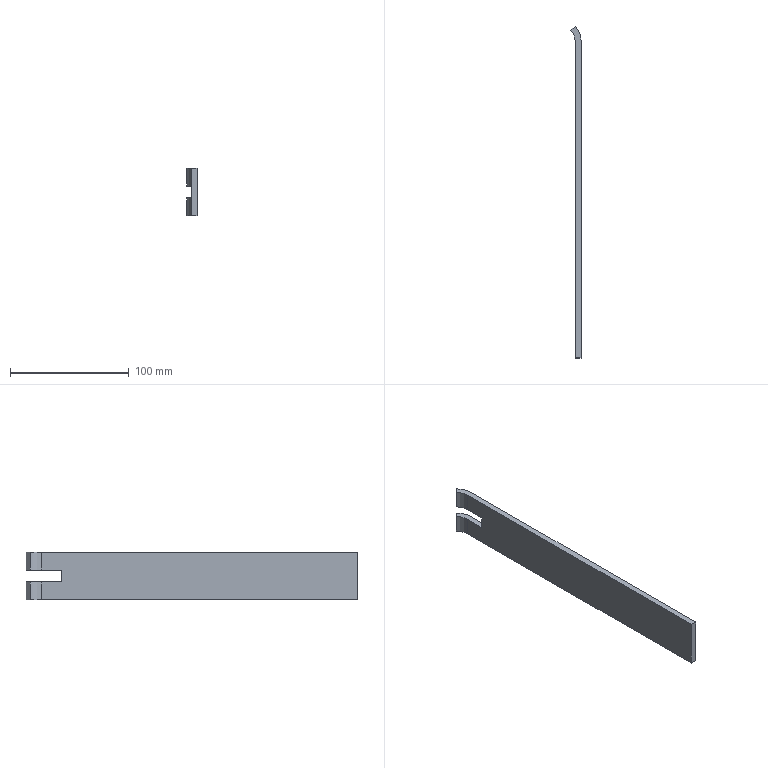Part | SolidWorks | features ICE 2, Extrusion 1 | 1 solid | 14 faces | box 8.684 x 279.845 x 40 mm | volume 54380 mm3 | plane 10 | cylinder 4 | commonest cylinder face diameters 28 x2 38 x2
STEP:
#1=CARTESIAN_POINT('',(0.,273.845,15.));
#2=VERTEX_POINT('',#1);
#3=CARTESIAN_POINT('',(0.,273.845,0.));
#4=VERTEX_POINT('',#3);
#5=CARTESIAN_POINT('',(0.,273.845,40.));
#6=DIRECTION('',(0.,0.,-1.));
#7=VECTOR('',#6,1000.);
#8=LINE('',#5,#7);
#9=EDGE_CURVE('',#2,#4,#8,.T.);
#10=ORIENTED_EDGE('',*,*,#9,.F.);
#11=CARTESIAN_POINT('',(5.,261.,15.));
#12=VERTEX_POINT('',#11);
#13=CARTESIAN_POINT('',(-14.,261.,15.));
#14=DIRECTION('',(0.,0.,-1.));
#15=DIRECTION('',(0.,1.,0.));
#16=AXIS2_PLACEMENT_3D('',#13,#14,#15);
#17=CIRCLE('',#16,19.);
#18=EDGE_CURVE('',#2,#12,#17,.T.);
#19=ORIENTED_EDGE('',*,*,#18,.T.);
#20=CARTESIAN_POINT('',(5.,261.,0.));
#21=VERTEX_POINT('',#20);
#22=CARTESIAN_POINT('',(5.,261.,40.));
#23=DIRECTION('',(0.,0.,-1.));
#24=VECTOR('',#23,1000.);
#25=LINE('',#22,#24);
#26=EDGE_CURVE('',#12,#21,#25,.T.);
#27=ORIENTED_EDGE('',*,*,#26,.T.);
#28=CARTESIAN_POINT('',(-14.,261.,0.));
#29=DIRECTION('',(0.,0.,1.));
#30=DIRECTION('',(1.,0.,0.));
#31=AXIS2_PLACEMENT_3D('',#28,#29,#30);
#32=CIRCLE('',#31,19.);
#33=EDGE_CURVE('',#21,#4,#32,.T.);
#34=ORIENTED_EDGE('',*,*,#33,.T.);
#35=EDGE_LOOP('',(#10,#19,#27,#34));
#36=FACE_OUTER_BOUND('',#35,.T.);
#37=CARTESIAN_POINT('',(-14.,261.,40.));
#38=DIRECTION('',(0.,0.,-1.));
#39=DIRECTION('',(-1.,0.,0.));
#40=AXIS2_PLACEMENT_3D('',#37,#38,#39);
#41=CYLINDRICAL_SURFACE('',#40,19.);
#42=ADVANCED_FACE('',(#36),#41,.T.);
#43=CARTESIAN_POINT('',(-3.684,270.465,15.));
#44=VERTEX_POINT('',#43);
#45=CARTESIAN_POINT('',(-3.684,270.465,0.));
#46=VERTEX_POINT('',#45);
#47=CARTESIAN_POINT('',(-3.684,270.465,40.));
#48=DIRECTION('',(0.,0.,-1.));
#49=VECTOR('',#48,1000.);
#50=LINE('',#47,#49);
#51=EDGE_CURVE('',#44,#46,#50,.T.);
#52=ORIENTED_EDGE('',*,*,#51,.F.);
#53=CARTESIAN_POINT('',(-3.684,270.465,15.));
#54=DIRECTION('',(0.7368,0.6761,0.));
#55=VECTOR('',#54,1000.);
#56=LINE('',#53,#55);
#57=EDGE_CURVE('',#44,#2,#56,.T.);
#58=ORIENTED_EDGE('',*,*,#57,.T.);
#59=ORIENTED_EDGE('',*,*,#9,.T.);
#60=CARTESIAN_POINT('',(-3.684,270.465,0.));
#61=DIRECTION('',(-0.7368,-0.6761,0.));
#62=VECTOR('',#61,1000.);
#63=LINE('',#60,#62);
#64=EDGE_CURVE('',#4,#46,#63,.T.);
#65=ORIENTED_EDGE('',*,*,#64,.T.);
#66=EDGE_LOOP('',(#52,#58,#59,#65));
#67=FACE_OUTER_BOUND('',#66,.T.);
#68=CARTESIAN_POINT('',(-3.684,270.465,40.));
#69=DIRECTION('',(0.6761,-0.7368,0.));
#70=DIRECTION('',(0.7368,0.6761,0.));
#71=AXIS2_PLACEMENT_3D('',#68,#69,#70);
#72=PLANE('',#71);
#73=ADVANCED_FACE('',(#67),#72,.F.);
#74=CARTESIAN_POINT('',(0.,261.,15.));
#75=VERTEX_POINT('',#74);
#76=CARTESIAN_POINT('',(0.,261.,0.));
#77=VERTEX_POINT('',#76);
#78=CARTESIAN_POINT('',(0.,261.,40.));
#79=DIRECTION('',(0.,0.,-1.));
#80=VECTOR('',#79,1000.);
#81=LINE('',#78,#80);
#82=EDGE_CURVE('',#75,#77,#81,.T.);
#83=ORIENTED_EDGE('',*,*,#82,.F.);
#84=CARTESIAN_POINT('',(-14.,261.,15.));
#85=DIRECTION('',(0.,0.,1.));
#86=DIRECTION('',(0.,1.,0.));
#87=AXIS2_PLACEMENT_3D('',#84,#85,#86);
#88=CIRCLE('',#87,14.);
#89=EDGE_CURVE('',#75,#44,#88,.T.);
#90=ORIENTED_EDGE('',*,*,#89,.T.);
#91=ORIENTED_EDGE('',*,*,#51,.T.);
#92=CARTESIAN_POINT('',(-14.,261.,0.));
#93=DIRECTION('',(0.,0.,-1.));
#94=DIRECTION('',(1.,0.,0.));
#95=AXIS2_PLACEMENT_3D('',#92,#93,#94);
#96=CIRCLE('',#95,14.);
#97=EDGE_CURVE('',#46,#77,#96,.T.);
#98=ORIENTED_EDGE('',*,*,#97,.T.);
#99=EDGE_LOOP('',(#83,#90,#91,#98));
#100=FACE_OUTER_BOUND('',#99,.T.);
#101=CARTESIAN_POINT('',(-14.,261.,40.));
#102=DIRECTION('',(0.,0.,-1.));
#103=DIRECTION('',(-1.,0.,0.));
#104=AXIS2_PLACEMENT_3D('',#101,#102,#103);
#105=CYLINDRICAL_SURFACE('',#104,14.);
#106=ADVANCED_FACE('',(#100),#105,.F.);
#107=CARTESIAN_POINT('',(0.,243.845,25.));
#108=VERTEX_POINT('',#107);
#109=CARTESIAN_POINT('',(0.,243.845,15.));
#110=VERTEX_POINT('',#109);
#111=CARTESIAN_POINT('',(0.,243.845,40.));
#112=DIRECTION('',(0.,0.,-1.));
#113=VECTOR('',#112,1000.);
#114=LINE('',#111,#113);
#115=EDGE_CURVE('',#108,#110,#114,.T.);
#116=ORIENTED_EDGE('',*,*,#115,.T.);
#117=CARTESIAN_POINT('',(0.,0.,15.));
#118=DIRECTION('',(0.,1.,0.));
#119=VECTOR('',#118,1000.);
#120=LINE('',#117,#119);
#121=EDGE_CURVE('',#110,#75,#120,.T.);
#122=ORIENTED_EDGE('',*,*,#121,.T.);
#123=ORIENTED_EDGE('',*,*,#82,.T.);
#124=CARTESIAN_POINT('',(0.,-6.,0.));
#125=VERTEX_POINT('',#124);
#126=CARTESIAN_POINT('',(0.,0.,0.));
#127=DIRECTION('',(0.,-1.,0.));
#128=VECTOR('',#127,1000.);
#129=LINE('',#126,#128);
#130=EDGE_CURVE('',#77,#125,#129,.T.);
#131=ORIENTED_EDGE('',*,*,#130,.T.);
#132=CARTESIAN_POINT('',(0.,-6.,40.));
#133=VERTEX_POINT('',#132);
#134=CARTESIAN_POINT('',(0.,-6.,40.));
#135=DIRECTION('',(0.,0.,-1.));
#136=VECTOR('',#135,1000.);
#137=LINE('',#134,#136);
#138=EDGE_CURVE('',#133,#125,#137,.T.);
#139=ORIENTED_EDGE('',*,*,#138,.F.);
#140=CARTESIAN_POINT('',(0.,261.,40.));
#141=VERTEX_POINT('',#140);
#142=CARTESIAN_POINT('',(0.,0.,40.));
#143=DIRECTION('',(0.,-1.,0.));
#144=VECTOR('',#143,1000.);
#145=LINE('',#142,#144);
#146=EDGE_CURVE('',#141,#133,#145,.T.);
#147=ORIENTED_EDGE('',*,*,#146,.F.);
#148=CARTESIAN_POINT('',(0.,261.,25.));
#149=VERTEX_POINT('',#148);
#150=CARTESIAN_POINT('',(0.,261.,40.));
#151=DIRECTION('',(0.,0.,-1.));
#152=VECTOR('',#151,1000.);
#153=LINE('',#150,#152);
#154=EDGE_CURVE('',#141,#149,#153,.T.);
#155=ORIENTED_EDGE('',*,*,#154,.T.);
#156=CARTESIAN_POINT('',(0.,0.,25.));
#157=DIRECTION('',(0.,-1.,0.));
#158=VECTOR('',#157,1000.);
#159=LINE('',#156,#158);
#160=EDGE_CURVE('',#149,#108,#159,.T.);
#161=ORIENTED_EDGE('',*,*,#160,.T.);
#162=EDGE_LOOP('',(#116,#122,#123,#131,#139,#147,#155,#161));
#163=FACE_OUTER_BOUND('',#162,.T.);
#164=CARTESIAN_POINT('',(0.,0.,40.));
#165=DIRECTION('',(1.,0.,0.));
#166=DIRECTION('',(0.,1.,0.));
#167=AXIS2_PLACEMENT_3D('',#164,#165,#166);
#168=PLANE('',#167);
#169=ADVANCED_FACE('',(#163),#168,.F.);
#170=ORIENTED_EDGE('',*,*,#26,.F.);
#171=CARTESIAN_POINT('',(5.,243.845,15.));
#172=VERTEX_POINT('',#171);
#173=CARTESIAN_POINT('',(5.,273.845,15.));
#174=DIRECTION('',(0.,1.,0.));
#175=VECTOR('',#174,1000.);
#176=LINE('',#173,#175);
#177=EDGE_CURVE('',#172,#12,#176,.T.);
#178=ORIENTED_EDGE('',*,*,#177,.F.);
#179=CARTESIAN_POINT('',(5.,243.845,25.));
#180=VERTEX_POINT('',#179);
#181=CARTESIAN_POINT('',(5.,243.845,15.));
#182=DIRECTION('',(0.,0.,-1.));
#183=VECTOR('',#182,1000.);
#184=LINE('',#181,#183);
#185=EDGE_CURVE('',#180,#172,#184,.T.);
#186=ORIENTED_EDGE('',*,*,#185,.F.);
#187=CARTESIAN_POINT('',(5.,261.,25.));
#188=VERTEX_POINT('',#187);
#189=CARTESIAN_POINT('',(5.,243.845,25.));
#190=DIRECTION('',(0.,-1.,0.));
#191=VECTOR('',#190,1000.);
#192=LINE('',#189,#191);
#193=EDGE_CURVE('',#188,#180,#192,.T.);
#194=ORIENTED_EDGE('',*,*,#193,.F.);
#195=CARTESIAN_POINT('',(5.,261.,40.));
#196=VERTEX_POINT('',#195);
#197=CARTESIAN_POINT('',(5.,261.,40.));
#198=DIRECTION('',(0.,0.,-1.));
#199=VECTOR('',#198,1000.);
#200=LINE('',#197,#199);
#201=EDGE_CURVE('',#196,#188,#200,.T.);
#202=ORIENTED_EDGE('',*,*,#201,.F.);
#203=CARTESIAN_POINT('',(5.,-6.,40.));
#204=VERTEX_POINT('',#203);
#205=CARTESIAN_POINT('',(5.,0.,40.));
#206=DIRECTION('',(0.,1.,0.));
#207=VECTOR('',#206,1000.);
#208=LINE('',#205,#207);
#209=EDGE_CURVE('',#204,#196,#208,.T.);
#210=ORIENTED_EDGE('',*,*,#209,.F.);
#211=CARTESIAN_POINT('',(5.,-6.,0.));
#212=VERTEX_POINT('',#211);
#213=CARTESIAN_POINT('',(5.,-6.,0.));
#214=DIRECTION('',(0.,0.,1.));
#215=VECTOR('',#214,1000.);
#216=LINE('',#213,#215);
#217=EDGE_CURVE('',#212,#204,#216,.T.);
#218=ORIENTED_EDGE('',*,*,#217,.F.);
#219=CARTESIAN_POINT('',(5.,0.,0.));
#220=DIRECTION('',(0.,1.,0.));
#221=VECTOR('',#220,1000.);
#222=LINE('',#219,#221);
#223=EDGE_CURVE('',#212,#21,#222,.T.);
#224=ORIENTED_EDGE('',*,*,#223,.T.);
#225=EDGE_LOOP('',(#170,#178,#186,#194,#202,#210,#218,#224));
#226=FACE_OUTER_BOUND('',#225,.T.);
#227=CARTESIAN_POINT('',(5.,0.,40.));
#228=DIRECTION('',(-1.,0.,0.));
#229=DIRECTION('',(0.,0.,1.));
#230=AXIS2_PLACEMENT_3D('',#227,#228,#229);
#231=PLANE('',#230);
#232=ADVANCED_FACE('',(#226),#231,.F.);
#233=ORIENTED_EDGE('',*,*,#201,.T.);
#234=CARTESIAN_POINT('',(0.,273.845,25.));
#235=VERTEX_POINT('',#234);
#236=CARTESIAN_POINT('',(-14.,261.,25.));
#237=DIRECTION('',(0.,0.,1.));
#238=DIRECTION('',(1.,0.,0.));
#239=AXIS2_PLACEMENT_3D('',#236,#237,#238);
#240=CIRCLE('',#239,19.);
#241=EDGE_CURVE('',#188,#235,#240,.T.);
#242=ORIENTED_EDGE('',*,*,#241,.T.);
#243=CARTESIAN_POINT('',(0.,273.845,40.));
#244=VERTEX_POINT('',#243);
#245=CARTESIAN_POINT('',(0.,273.845,40.));
#246=DIRECTION('',(0.,0.,-1.));
#247=VECTOR('',#246,1000.);
#248=LINE('',#245,#247);
#249=EDGE_CURVE('',#244,#235,#248,.T.);
#250=ORIENTED_EDGE('',*,*,#249,.F.);
#251=CARTESIAN_POINT('',(-14.,261.,40.));
#252=DIRECTION('',(0.,0.,1.));
#253=DIRECTION('',(1.,0.,0.));
#254=AXIS2_PLACEMENT_3D('',#251,#252,#253);
#255=CIRCLE('',#254,19.);
#256=EDGE_CURVE('',#196,#244,#255,.T.);
#257=ORIENTED_EDGE('',*,*,#256,.F.);
#258=EDGE_LOOP('',(#233,#242,#250,#257));
#259=FACE_OUTER_BOUND('',#258,.T.);
#260=CARTESIAN_POINT('',(-14.,261.,40.));
#261=DIRECTION('',(0.,0.,-1.));
#262=DIRECTION('',(-1.,0.,0.));
#263=AXIS2_PLACEMENT_3D('',#260,#261,#262);
#264=CYLINDRICAL_SURFACE('',#263,19.);
#265=ADVANCED_FACE('',(#259),#264,.T.);
#266=ORIENTED_EDGE('',*,*,#249,.T.);
#267=CARTESIAN_POINT('',(-3.684,270.465,25.));
#268=VERTEX_POINT('',#267);
#269=CARTESIAN_POINT('',(-3.684,270.465,25.));
#270=DIRECTION('',(-0.7368,-0.6761,0.));
#271=VECTOR('',#270,1000.);
#272=LINE('',#269,#271);
#273=EDGE_CURVE('',#235,#268,#272,.T.);
#274=ORIENTED_EDGE('',*,*,#273,.T.);
#275=CARTESIAN_POINT('',(-3.684,270.465,40.));
#276=VERTEX_POINT('',#275);
#277=CARTESIAN_POINT('',(-3.684,270.465,40.));
#278=DIRECTION('',(0.,0.,-1.));
#279=VECTOR('',#278,1000.);
#280=LINE('',#277,#279);
#281=EDGE_CURVE('',#276,#268,#280,.T.);
#282=ORIENTED_EDGE('',*,*,#281,.F.);
#283=CARTESIAN_POINT('',(-3.684,270.465,40.));
#284=DIRECTION('',(-0.7368,-0.6761,0.));
#285=VECTOR('',#284,1000.);
#286=LINE('',#283,#285);
#287=EDGE_CURVE('',#244,#276,#286,.T.);
#288=ORIENTED_EDGE('',*,*,#287,.F.);
#289=EDGE_LOOP('',(#266,#274,#282,#288));
#290=FACE_OUTER_BOUND('',#289,.T.);
#291=CARTESIAN_POINT('',(-3.684,270.465,40.));
#292=DIRECTION('',(0.6761,-0.7368,0.));
#293=DIRECTION('',(0.7368,0.6761,0.));
#294=AXIS2_PLACEMENT_3D('',#291,#292,#293);
#295=PLANE('',#294);
#296=ADVANCED_FACE('',(#290),#295,.F.);
#297=ORIENTED_EDGE('',*,*,#281,.T.);
#298=CARTESIAN_POINT('',(-14.,261.,25.));
#299=DIRECTION('',(0.,0.,-1.));
#300=DIRECTION('',(1.,0.,0.));
#301=AXIS2_PLACEMENT_3D('',#298,#299,#300);
#302=CIRCLE('',#301,14.);
#303=EDGE_CURVE('',#268,#149,#302,.T.);
#304=ORIENTED_EDGE('',*,*,#303,.T.);
#305=ORIENTED_EDGE('',*,*,#154,.F.);
#306=CARTESIAN_POINT('',(-14.,261.,40.));
#307=DIRECTION('',(0.,0.,-1.));
#308=DIRECTION('',(1.,0.,0.));
#309=AXIS2_PLACEMENT_3D('',#306,#307,#308);
#310=CIRCLE('',#309,14.);
#311=EDGE_CURVE('',#276,#141,#310,.T.);
#312=ORIENTED_EDGE('',*,*,#311,.F.);
#313=EDGE_LOOP('',(#297,#304,#305,#312));
#314=FACE_OUTER_BOUND('',#313,.T.);
#315=CARTESIAN_POINT('',(-14.,261.,40.));
#316=DIRECTION('',(0.,0.,-1.));
#317=DIRECTION('',(-1.,0.,0.));
#318=AXIS2_PLACEMENT_3D('',#315,#316,#317);
#319=CYLINDRICAL_SURFACE('',#318,14.);
#320=ADVANCED_FACE('',(#314),#319,.F.);
#321=ORIENTED_EDGE('',*,*,#146,.T.);
#322=CARTESIAN_POINT('',(5.,-6.,40.));
#323=DIRECTION('',(-1.,0.,0.));
#324=VECTOR('',#323,1000.);
#325=LINE('',#322,#324);
#326=EDGE_CURVE('',#204,#133,#325,.T.);
#327=ORIENTED_EDGE('',*,*,#326,.F.);
#328=ORIENTED_EDGE('',*,*,#209,.T.);
#329=ORIENTED_EDGE('',*,*,#256,.T.);
#330=ORIENTED_EDGE('',*,*,#287,.T.);
#331=ORIENTED_EDGE('',*,*,#311,.T.);
#332=EDGE_LOOP('',(#321,#327,#328,#329,#330,#331));
#333=FACE_OUTER_BOUND('',#332,.T.);
#334=CARTESIAN_POINT('',(-14.,261.,40.));
#335=DIRECTION('',(0.,0.,1.));
#336=DIRECTION('',(1.,0.,0.));
#337=AXIS2_PLACEMENT_3D('',#334,#335,#336);
#338=PLANE('',#337);
#339=ADVANCED_FACE('',(#333),#338,.T.);
#340=ORIENTED_EDGE('',*,*,#130,.F.);
#341=ORIENTED_EDGE('',*,*,#97,.F.);
#342=ORIENTED_EDGE('',*,*,#64,.F.);
#343=ORIENTED_EDGE('',*,*,#33,.F.);
#344=ORIENTED_EDGE('',*,*,#223,.F.);
#345=CARTESIAN_POINT('',(0.,-6.,0.));
#346=DIRECTION('',(1.,0.,0.));
#347=VECTOR('',#346,1000.);
#348=LINE('',#345,#347);
#349=EDGE_CURVE('',#125,#212,#348,.T.);
#350=ORIENTED_EDGE('',*,*,#349,.F.);
#351=EDGE_LOOP('',(#340,#341,#342,#343,#344,#350));
#352=FACE_OUTER_BOUND('',#351,.T.);
#353=CARTESIAN_POINT('',(-14.,261.,0.));
#354=DIRECTION('',(0.,0.,1.));
#355=DIRECTION('',(1.,0.,0.));
#356=AXIS2_PLACEMENT_3D('',#353,#354,#355);
#357=PLANE('',#356);
#358=ADVANCED_FACE('',(#352),#357,.F.);
#359=CARTESIAN_POINT('',(-35.,243.845,25.));
#360=DIRECTION('',(1.,0.,0.));
#361=VECTOR('',#360,1000.);
#362=LINE('',#359,#361);
#363=EDGE_CURVE('',#108,#180,#362,.T.);
#364=ORIENTED_EDGE('',*,*,#363,.T.);
#365=ORIENTED_EDGE('',*,*,#185,.T.);
#366=CARTESIAN_POINT('',(-35.,243.845,15.));
#367=DIRECTION('',(1.,0.,0.));
#368=VECTOR('',#367,1000.);
#369=LINE('',#366,#368);
#370=EDGE_CURVE('',#110,#172,#369,.T.);
#371=ORIENTED_EDGE('',*,*,#370,.F.);
#372=ORIENTED_EDGE('',*,*,#115,.F.);
#373=EDGE_LOOP('',(#364,#365,#371,#372));
#374=FACE_OUTER_BOUND('',#373,.T.);
#375=CARTESIAN_POINT('',(-35.,243.845,15.));
#376=DIRECTION('',(0.,-1.,0.));
#377=DIRECTION('',(0.,0.,-1.));
#378=AXIS2_PLACEMENT_3D('',#375,#376,#377);
#379=PLANE('',#378);
#380=ADVANCED_FACE('',(#374),#379,.F.);
#381=ORIENTED_EDGE('',*,*,#370,.T.);
#382=ORIENTED_EDGE('',*,*,#177,.T.);
#383=ORIENTED_EDGE('',*,*,#18,.F.);
#384=ORIENTED_EDGE('',*,*,#57,.F.);
#385=ORIENTED_EDGE('',*,*,#89,.F.);
#386=ORIENTED_EDGE('',*,*,#121,.F.);
#387=EDGE_LOOP('',(#381,#382,#383,#384,#385,#386));
#388=FACE_OUTER_BOUND('',#387,.T.);
#389=CARTESIAN_POINT('',(-35.,273.845,15.));
#390=DIRECTION('',(0.,0.,-1.));
#391=DIRECTION('',(0.,1.,0.));
#392=AXIS2_PLACEMENT_3D('',#389,#390,#391);
#393=PLANE('',#392);
#394=ADVANCED_FACE('',(#388),#393,.F.);
#395=ORIENTED_EDGE('',*,*,#303,.F.);
#396=ORIENTED_EDGE('',*,*,#273,.F.);
#397=ORIENTED_EDGE('',*,*,#241,.F.);
#398=ORIENTED_EDGE('',*,*,#193,.T.);
#399=ORIENTED_EDGE('',*,*,#363,.F.);
#400=ORIENTED_EDGE('',*,*,#160,.F.);
#401=EDGE_LOOP('',(#395,#396,#397,#398,#399,#400));
#402=FACE_OUTER_BOUND('',#401,.T.);
#403=CARTESIAN_POINT('',(-35.,243.845,25.));
#404=DIRECTION('',(0.,0.,1.));
#405=DIRECTION('',(1.,0.,0.));
#406=AXIS2_PLACEMENT_3D('',#403,#404,#405);
#407=PLANE('',#406);
#408=ADVANCED_FACE('',(#402),#407,.F.);
#409=ORIENTED_EDGE('',*,*,#138,.T.);
#410=ORIENTED_EDGE('',*,*,#349,.T.);
#411=ORIENTED_EDGE('',*,*,#217,.T.);
#412=ORIENTED_EDGE('',*,*,#326,.T.);
#413=EDGE_LOOP('',(#409,#410,#411,#412));
#414=FACE_OUTER_BOUND('',#413,.T.);
#415=CARTESIAN_POINT('',(0.,-6.,0.));
#416=DIRECTION('',(0.,-1.,0.));
#417=DIRECTION('',(0.,0.,-1.));
#418=AXIS2_PLACEMENT_3D('',#415,#416,#417);
#419=PLANE('',#418);
#420=ADVANCED_FACE('',(#414),#419,.T.);
#421=CLOSED_SHELL('',(#42,#73,#106,#169,#232,#265,#296,#320,#339,#358,#380,#394,#408,#420));
#422=MANIFOLD_SOLID_BREP('',#421);
#423=CARTESIAN_POINT('',(0.,0.,0.));
#424=DIRECTION('',(0.,0.,1.));
#425=DIRECTION('',(1.,0.,0.));
#426=AXIS2_PLACEMENT_3D('',#423,#424,#425);
#427=(LENGTH_UNIT()NAMED_UNIT(*)SI_UNIT(.MILLI.,.METRE.));
#428=UNCERTAINTY_MEASURE_WITH_UNIT(LENGTH_MEASURE(0.00001),#427,'','');
#429=(NAMED_UNIT(*)PLANE_ANGLE_UNIT()SI_UNIT($,.RADIAN.));
#430=(NAMED_UNIT(*)SI_UNIT($,.STERADIAN.)SOLID_ANGLE_UNIT());
#431=(GEOMETRIC_REPRESENTATION_CONTEXT(3)GLOBAL_UNCERTAINTY_ASSIGNED_CONTEXT((#428))GLOBAL_UNIT_ASSIGNED_CONTEXT((#427,#429,#430))REPRESENTATION_CONTEXT('',''));
#432=ADVANCED_BREP_SHAPE_REPRESENTATION('',(#422,#426),#431);